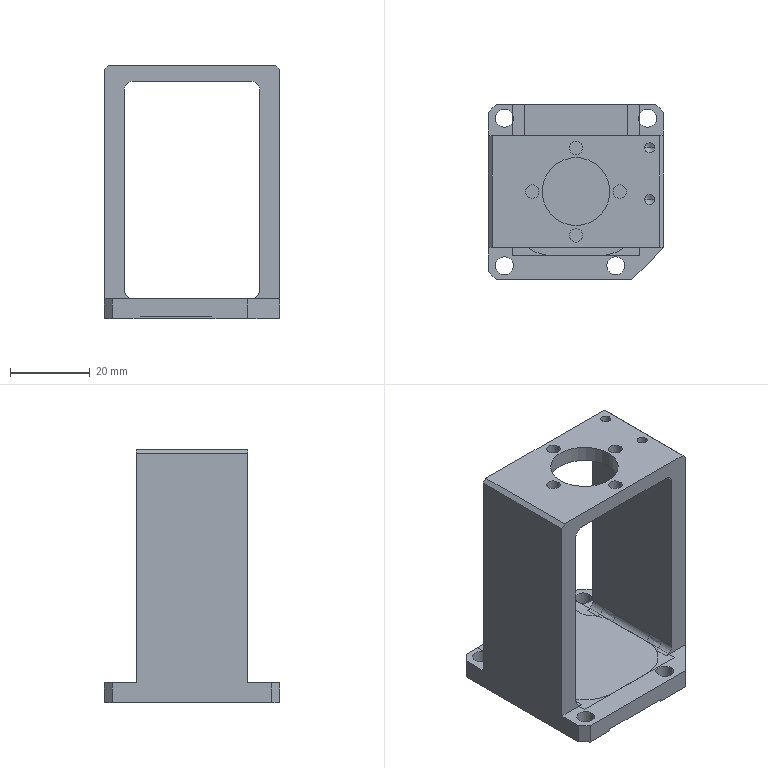NC program | NX | posted with a generic post | part box 44 x 44 x 63.6 mm
Lines 62 to 1050 of 4011:
(ZLEVEL_PROFILE , TOOL : D20)
N104 T02 M6
N106 G54
N108 G17 G0 G90 X0.611 Y32.1 B0. C0. S9500 M3
N110 G43 Z30. H2
N112 Z1.5
N114 G94 G1 X20.779 Z0.443 F1000.
N116 X22.872 Y31.714 Z0.332
N118 X24.838 Y30.9 Z0.22
N120 X26.591 Y29.693 Z0.108
N122 X29.693 Y26.591 Z-0.121
N124 X30.9 Y24.838 Z-0.233
N126 X31.714 Y22.872 Z-0.345
N128 X32.1 Y20.779 Z-0.456
N130 Y20. Z-0.497
N132 Y-20. F3000.
N134 G2 X29.142 Y-27.142 R10.1
N136 G1 X27.142 Y-29.142
N138 G2 X20. Y-32.1 R10.1
N140 G1 X-20.
N142 G2 X-27.142 Y-29.142 R10.1
N144 G1 X-29.142 Y-27.142
N146 G2 X-32.1 Y-20. R10.1
N148 G1 Y14.
N150 G2 X-29.142 Y21.142 R10.1
N152 G1 X-21.142 Y29.142
N154 G2 X-14. Y32.1 R10.1
N156 G1 X20.
N158 G2 X27.142 Y29.142 R10.1
N160 G1 X29.142 Y27.142
N162 G2 X32.1 Y20. R10.1
N164 G1 Y-8.466 Z-0.994
N166 Y-20.
N168 G2 X29.142 Y-27.142 R10.1
N170 G1 X27.142 Y-29.142
N172 G2 X20. Y-32.1 R10.1
N174 G1 X-20.
N176 G2 X-27.142 Y-29.142 R10.1
N178 G1 X-29.142 Y-27.142
N180 G2 X-32.1 Y-20. R10.1
N182 G1 Y14.
N184 G2 X-29.142 Y21.142 R10.1
N186 G1 X-21.142 Y29.142
N188 G2 X-14. Y32.1 R10.1
N190 G1 X20.
N192 G2 X27.142 Y29.142 R10.1
N194 G1 X29.142 Y27.142
N196 G2 X32.1 Y20. R10.1
N198 G1 Y-8.466 Z-1.491
N200 Y-20.
N202 G2 X29.142 Y-27.142 R10.1
N204 G1 X27.142 Y-29.142
N206 G2 X20. Y-32.1 R10.1
N208 G1 X-20.
N210 G2 X-27.142 Y-29.142 R10.1
N212 G1 X-29.142 Y-27.142
N214 G2 X-32.1 Y-20. R10.1
N216 G1 Y14.
N218 G2 X-29.142 Y21.142 R10.1
N220 G1 X-21.142 Y29.142
N222 G2 X-14. Y32.1 R10.1
N224 G1 X20.
N226 G2 X27.142 Y29.142 R10.1
N228 G1 X29.142 Y27.142
N230 G2 X32.1 Y20. R10.1
N232 G1 Y-8.466 Z-1.988
N234 Y-20.
N236 G2 X29.142 Y-27.142 R10.1
N238 G1 X27.142 Y-29.142
N240 G2 X20. Y-32.1 R10.1
N242 G1 X-20.
N244 G2 X-27.142 Y-29.142 R10.1
N246 G1 X-29.142 Y-27.142
N248 G2 X-32.1 Y-20. R10.1
N250 G1 Y14.
N252 G2 X-29.142 Y21.142 R10.1
N254 G1 X-21.142 Y29.142
N256 G2 X-14. Y32.1 R10.1
N258 G1 X20.
N260 G2 X27.142 Y29.142 R10.1
N262 G1 X29.142 Y27.142
N264 G2 X32.1 Y20. R10.1
N266 G1 Y-8.466 Z-2.484
N268 Y-20.
N270 G2 X29.142 Y-27.142 R10.1
N272 G1 X27.142 Y-29.142
N274 G2 X20. Y-32.1 R10.1
N276 G1 X-20.
N278 G2 X-27.142 Y-29.142 R10.1
N280 G1 X-29.142 Y-27.142
N282 G2 X-32.1 Y-20. R10.1
N284 G1 Y14.
N286 G2 X-29.142 Y21.142 R10.1
N288 G1 X-21.142 Y29.142
N290 G2 X-14. Y32.1 R10.1
N292 G1 X20.
N294 G2 X27.142 Y29.142 R10.1
N296 G1 X29.142 Y27.142
N298 G2 X32.1 Y20. R10.1
N300 G1 Y-8.466 Z-2.981
N302 Y-20.
N304 G2 X29.142 Y-27.142 R10.1
N306 G1 X27.142 Y-29.142
N308 G2 X20. Y-32.1 R10.1
N310 G1 X-20.
N312 G2 X-27.142 Y-29.142 R10.1
N314 G1 X-29.142 Y-27.142
N316 G2 X-32.1 Y-20. R10.1
N318 G1 Y14.
N320 G2 X-29.142 Y21.142 R10.1
N322 G1 X-21.142 Y29.142
N324 G2 X-14. Y32.1 R10.1
N326 G1 X20.
N328 G2 X27.142 Y29.142 R10.1
N330 G1 X29.142 Y27.142
N332 G2 X32.1 Y20. R10.1
N334 G1 Y-8.466 Z-3.478
N336 Y-20.
N338 G2 X29.142 Y-27.142 R10.1
N340 G1 X27.142 Y-29.142
N342 G2 X20. Y-32.1 R10.1
N344 G1 X-20.
N346 G2 X-27.142 Y-29.142 R10.1
N348 G1 X-29.142 Y-27.142
N350 G2 X-32.1 Y-20. R10.1
N352 G1 Y14.
N354 G2 X-29.142 Y21.142 R10.1
N356 G1 X-21.142 Y29.142
N358 G2 X-14. Y32.1 R10.1
N360 G1 X20.
N362 G2 X27.142 Y29.142 R10.1
N364 G1 X29.142 Y27.142
N366 G2 X32.1 Y20. R10.1
N368 G1 Y-8.466 Z-3.975
N370 Y-20.
N372 G2 X29.142 Y-27.142 R10.1
N374 G1 X27.142 Y-29.142
N376 G2 X20. Y-32.1 R10.1
N378 G1 X-20.
N380 G2 X-27.142 Y-29.142 R10.1
N382 G1 X-29.142 Y-27.142
N384 G2 X-32.1 Y-20. R10.1
N386 G1 Y14.
N388 G2 X-29.142 Y21.142 R10.1
N390 G1 X-21.142 Y29.142
N392 G2 X-14. Y32.1 R10.1
N394 G1 X20.
N396 G2 X27.142 Y29.142 R10.1
N398 G1 X29.142 Y27.142
N400 G2 X32.1 Y20. R10.1
N402 G1 Y-8.466 Z-4.472
N404 Y-20.
N406 G2 X29.142 Y-27.142 R10.1
N408 G1 X27.142 Y-29.142
N410 G2 X20. Y-32.1 R10.1
N412 G1 X-20.
N414 G2 X-27.142 Y-29.142 R10.1
N416 G1 X-29.142 Y-27.142
N418 G2 X-32.1 Y-20. R10.1
N420 G1 Y14.
N422 G2 X-29.142 Y21.142 R10.1
N424 G1 X-21.142 Y29.142
N426 G2 X-14. Y32.1 R10.1
N428 G1 X20.
N430 G2 X27.142 Y29.142 R10.1
N432 G1 X29.142 Y27.142
N434 G2 X32.1 Y20. R10.1
N436 G1 Y-8.466 Z-4.969
N438 Y-20.
N440 G2 X29.142 Y-27.142 R10.1
N442 G1 X27.142 Y-29.142
N444 G2 X20. Y-32.1 R10.1
N446 G1 X-20.
N448 G2 X-27.142 Y-29.142 R10.1
N450 G1 X-29.142 Y-27.142
N452 G2 X-32.1 Y-20. R10.1
N454 G1 Y14.
N456 G2 X-29.142 Y21.142 R10.1
N458 G1 X-21.142 Y29.142
N460 G2 X-14. Y32.1 R10.1
N462 G1 X20.
N464 G2 X27.142 Y29.142 R10.1
N466 G1 X29.142 Y27.142
N468 G2 X32.1 Y20. R10.1
N470 G1 Y-8.466 Z-5.466
N472 Y-20.
N474 G2 X29.142 Y-27.142 R10.1
N476 G1 X27.142 Y-29.142
N478 G2 X20. Y-32.1 R10.1
N480 G1 X-20.
N482 G2 X-27.142 Y-29.142 R10.1
N484 G1 X-29.142 Y-27.142
N486 G2 X-32.1 Y-20. R10.1
N488 G1 Y14.
N490 G2 X-29.142 Y21.142 R10.1
N492 G1 X-21.142 Y29.142
N494 G2 X-14. Y32.1 R10.1
N496 G1 X20.
N498 G2 X27.142 Y29.142 R10.1
N500 G1 X29.142 Y27.142
N502 G2 X32.1 Y20. R10.1
N504 G1 Y-8.466 Z-5.963
N506 Y-20.
N508 G2 X29.142 Y-27.142 R10.1
N510 G1 X27.142 Y-29.142
N512 G2 X20. Y-32.1 R10.1
N514 G1 X-20.
N516 G2 X-27.142 Y-29.142 R10.1
N518 G1 X-29.142 Y-27.142
N520 G2 X-32.1 Y-20. R10.1
N522 G1 Y14.
N524 G2 X-29.142 Y21.142 R10.1
N526 G1 X-21.142 Y29.142
N528 G2 X-14. Y32.1 R10.1
N530 G1 X20.
N532 G2 X27.142 Y29.142 R10.1
N534 G1 X29.142 Y27.142
N536 G2 X32.1 Y20. R10.1
N538 G1 Y-8.466 Z-6.459
N540 Y-20.
N542 G2 X29.142 Y-27.142 R10.1
N544 G1 X27.142 Y-29.142
N546 G2 X20. Y-32.1 R10.1
N548 G1 X-20.
N550 G2 X-27.142 Y-29.142 R10.1
N552 G1 X-29.142 Y-27.142
N554 G2 X-32.1 Y-20. R10.1
N556 G1 Y14.
N558 G2 X-29.142 Y21.142 R10.1
N560 G1 X-21.142 Y29.142
N562 G2 X-14. Y32.1 R10.1
N564 G1 X20.
N566 G2 X27.142 Y29.142 R10.1
N568 G1 X29.142 Y27.142
N570 G2 X32.1 Y20. R10.1
N572 G1 Y-8.466 Z-6.956
N574 Y-20.
N576 G2 X29.142 Y-27.142 R10.1
N578 G1 X27.142 Y-29.142
N580 G2 X20. Y-32.1 R10.1
N582 G1 X-20.
N584 G2 X-27.142 Y-29.142 R10.1
N586 G1 X-29.142 Y-27.142
N588 G2 X-32.1 Y-20. R10.1
N590 G1 Y14.
N592 G2 X-29.142 Y21.142 R10.1
N594 G1 X-21.142 Y29.142
N596 G2 X-14. Y32.1 R10.1
N598 G1 X20.
N600 G2 X27.142 Y29.142 R10.1
N602 G1 X29.142 Y27.142
N604 G2 X32.1 Y20. R10.1
N606 G1 Y-8.466 Z-7.453
N608 Y-20.
N610 G2 X29.142 Y-27.142 R10.1
N612 G1 X27.142 Y-29.142
N614 G2 X20. Y-32.1 R10.1
N616 G1 X-20.
N618 G2 X-27.142 Y-29.142 R10.1
N620 G1 X-29.142 Y-27.142
N622 G2 X-32.1 Y-20. R10.1
N624 G1 Y14.
N626 G2 X-29.142 Y21.142 R10.1
N628 G1 X-21.142 Y29.142
N630 G2 X-14. Y32.1 R10.1
N632 G1 X20.
N634 G2 X27.142 Y29.142 R10.1
N636 G1 X29.142 Y27.142
N638 G2 X32.1 Y20. R10.1
N640 G1 Y-8.466 Z-7.95
N642 Y-20.
N644 G2 X29.142 Y-27.142 R10.1
N646 G1 X27.142 Y-29.142
N648 G2 X20. Y-32.1 R10.1
N650 G1 X-20.
N652 G2 X-27.142 Y-29.142 R10.1
N654 G1 X-29.142 Y-27.142
N656 G2 X-32.1 Y-20. R10.1
N658 G1 Y14.
N660 G2 X-29.142 Y21.142 R10.1
N662 G1 X-21.142 Y29.142
N664 G2 X-14. Y32.1 R10.1
N666 G1 X20.
N668 G2 X27.142 Y29.142 R10.1
N670 G1 X29.142 Y27.142
N672 G2 X32.1 Y20. R10.1
N674 G1 Y-8.466 Z-8.447
N676 Y-20.
N678 G2 X29.142 Y-27.142 R10.1
N680 G1 X27.142 Y-29.142
N682 G2 X20. Y-32.1 R10.1
N684 G1 X-20.
N686 G2 X-27.142 Y-29.142 R10.1
N688 G1 X-29.142 Y-27.142
N690 G2 X-32.1 Y-20. R10.1
N692 G1 Y14.
N694 G2 X-29.142 Y21.142 R10.1
N696 G1 X-21.142 Y29.142
N698 G2 X-14. Y32.1 R10.1
N700 G1 X20.
N702 G2 X27.142 Y29.142 R10.1
N704 G1 X29.142 Y27.142
N706 G2 X32.1 Y20. R10.1
N708 G1 Y-8.466 Z-8.944
N710 Y-20.
N712 G2 X29.142 Y-27.142 R10.1
N714 G1 X27.142 Y-29.142
N716 G2 X20. Y-32.1 R10.1
N718 G1 X-20.
N720 G2 X-27.142 Y-29.142 R10.1
N722 G1 X-29.142 Y-27.142
N724 G2 X-32.1 Y-20. R10.1
N726 G1 Y14.
N728 G2 X-29.142 Y21.142 R10.1
N730 G1 X-21.142 Y29.142
N732 G2 X-14. Y32.1 R10.1
N734 G1 X20.
N736 G2 X27.142 Y29.142 R10.1
N738 G1 X29.142 Y27.142
N740 G2 X32.1 Y20. R10.1
N742 G1 Y-8.466 Z-9.441
N744 Y-20.
N746 G2 X29.142 Y-27.142 R10.1
N748 G1 X27.142 Y-29.142
N750 G2 X20. Y-32.1 R10.1
N752 G1 X-20.
N754 G2 X-27.142 Y-29.142 R10.1
N756 G1 X-29.142 Y-27.142
N758 G2 X-32.1 Y-20. R10.1
N760 G1 Y14.
N762 G2 X-29.142 Y21.142 R10.1
N764 G1 X-21.142 Y29.142
N766 G2 X-14. Y32.1 R10.1
N768 G1 X20.
N770 G2 X27.142 Y29.142 R10.1
N772 G1 X29.142 Y27.142
N774 G2 X32.1 Y20. R10.1
N776 G1 Y-8.466 Z-9.938
N778 Y-20.
N780 G2 X29.142 Y-27.142 R10.1
N782 G1 X27.142 Y-29.142
N784 G2 X20. Y-32.1 R10.1
N786 G1 X-20.
N788 G2 X-27.142 Y-29.142 R10.1
N790 G1 X-29.142 Y-27.142
N792 G2 X-32.1 Y-20. R10.1
N794 G1 Y14.
N796 G2 X-29.142 Y21.142 R10.1
N798 G1 X-21.142 Y29.142
N800 G2 X-14. Y32.1 R10.1
N802 G1 X20.
N804 G2 X27.142 Y29.142 R10.1
N806 G1 X29.142 Y27.142
N808 G2 X32.1 Y20. R10.1
N810 G1 Y-8.466 Z-10.434
N812 Y-20.
N814 G2 X29.142 Y-27.142 R10.1
N816 G1 X27.142 Y-29.142
N818 G2 X20. Y-32.1 R10.1
N820 G1 X-20.
N822 G2 X-27.142 Y-29.142 R10.1
N824 G1 X-29.142 Y-27.142
N826 G2 X-32.1 Y-20. R10.1
N828 G1 Y14.
N830 G2 X-29.142 Y21.142 R10.1
N832 G1 X-21.142 Y29.142
N834 G2 X-14. Y32.1 R10.1
N836 G1 X20.
N838 G2 X27.142 Y29.142 R10.1
N840 G1 X29.142 Y27.142
N842 G2 X32.1 Y20. R10.1
N844 G1 Y-8.466 Z-10.931
N846 Y-20.
N848 G2 X29.142 Y-27.142 R10.1
N850 G1 X27.142 Y-29.142
N852 G2 X20. Y-32.1 R10.1
N854 G1 X-20.
N856 G2 X-27.142 Y-29.142 R10.1
N858 G1 X-29.142 Y-27.142
N860 G2 X-32.1 Y-20. R10.1
N862 G1 Y14.
N864 G2 X-29.142 Y21.142 R10.1
N866 G1 X-21.142 Y29.142
N868 G2 X-14. Y32.1 R10.1
N870 G1 X20.
N872 G2 X27.142 Y29.142 R10.1
N874 G1 X29.142 Y27.142
N876 G2 X32.1 Y20. R10.1
N878 G1 Y-8.466 Z-11.428
N880 Y-20.
N882 G2 X29.142 Y-27.142 R10.1
N884 G1 X27.142 Y-29.142
N886 G2 X20. Y-32.1 R10.1
N888 G1 X-20.
N890 G2 X-27.142 Y-29.142 R10.1
N892 G1 X-29.142 Y-27.142
N894 G2 X-32.1 Y-20. R10.1
N896 G1 Y14.
N898 G2 X-29.142 Y21.142 R10.1
N900 G1 X-21.142 Y29.142
N902 G2 X-14. Y32.1 R10.1
N904 G1 X20.
N906 G2 X27.142 Y29.142 R10.1
N908 G1 X29.142 Y27.142
N910 G2 X32.1 Y20. R10.1
N912 G1 Y-8.466 Z-11.925
N914 Y-20.
N916 G2 X29.142 Y-27.142 R10.1
N918 G1 X27.142 Y-29.142
N920 G2 X20. Y-32.1 R10.1
N922 G1 X-20.
N924 G2 X-27.142 Y-29.142 R10.1
N926 G1 X-29.142 Y-27.142
N928 G2 X-32.1 Y-20. R10.1
N930 G1 Y14.
N932 G2 X-29.142 Y21.142 R10.1
N934 G1 X-21.142 Y29.142
N936 G2 X-14. Y32.1 R10.1
N938 G1 X20.
N940 G2 X27.142 Y29.142 R10.1
N942 G1 X29.142 Y27.142
N944 G2 X32.1 Y20. R10.1
N946 G1 Y-8.466 Z-12.422
N948 Y-20.
N950 G2 X29.142 Y-27.142 R10.1
N952 G1 X27.142 Y-29.142
N954 G2 X20. Y-32.1 R10.1
N956 G1 X-20.
N958 G2 X-27.142 Y-29.142 R10.1
N960 G1 X-29.142 Y-27.142
N962 G2 X-32.1 Y-20. R10.1
N964 G1 Y14.
N966 G2 X-29.142 Y21.142 R10.1
N968 G1 X-21.142 Y29.142
N970 G2 X-14. Y32.1 R10.1
N972 G1 X20.
N974 G2 X27.142 Y29.142 R10.1
N976 G1 X29.142 Y27.142
N978 G2 X32.1 Y20. R10.1
N980 G1 Y-8.466 Z-12.919
N982 Y-20.
N984 G2 X29.142 Y-27.142 R10.1
N986 G1 X27.142 Y-29.142
N988 G2 X20. Y-32.1 R10.1
N990 G1 X-20.
N992 G2 X-27.142 Y-29.142 R10.1
N994 G1 X-29.142 Y-27.142
N996 G2 X-32.1 Y-20. R10.1
N998 G1 Y14.
N1000 G2 X-29.142 Y21.142 R10.1
N1002 G1 X-21.142 Y29.142
N1004 G2 X-14. Y32.1 R10.1
N1006 G1 X20.
N1008 G2 X27.142 Y29.142 R10.1
N1010 G1 X29.142 Y27.142
N1012 G2 X32.1 Y20. R10.1
N1014 G1 Y-8.466 Z-13.416
N1016 Y-20.
N1018 G2 X29.142 Y-27.142 R10.1
N1020 G1 X27.142 Y-29.142
N1022 G2 X20. Y-32.1 R10.1
N1024 G1 X-20.
N1026 G2 X-27.142 Y-29.142 R10.1
N1028 G1 X-29.142 Y-27.142
N1030 G2 X-32.1 Y-20. R10.1
N1032 G1 Y14.
N1034 G2 X-29.142 Y21.142 R10.1
N1036 G1 X-21.142 Y29.142
N1038 G2 X-14. Y32.1 R10.1
N1040 G1 X20.
N1042 G2 X27.142 Y29.142 R10.1
N1044 G1 X29.142 Y27.142
N1046 G2 X32.1 Y20. R10.1
N1048 G1 Y-8.466 Z-13.913
N1050 Y-20.
N1052 G2 X29.142 Y-27.142 R10.1
N1054 G1 X27.142 Y-29.142
N1056 G2 X20. Y-32.1 R10.1
N1058 G1 X-20.
N1060 G2 X-27.142 Y-29.142 R10.1
N1062 G1 X-29.142 Y-27.142
N1064 G2 X-32.1 Y-20. R10.1
N1066 G1 Y14.
N1068 G2 X-29.142 Y21.142 R10.1
N1070 G1 X-21.142 Y29.142
N1072 G2 X-14. Y32.1 R10.1
N1074 G1 X20.
N1076 G2 X27.142 Y29.142 R10.1
N1078 G1 X29.142 Y27.142
N1080 G2 X32.1 Y20. R10.1
N1082 G1 Y-8.466 Z-14.409
N1084 Y-20.
N1086 G2 X29.142 Y-27.142 R10.1
N1088 G1 X27.142 Y-29.142
N1090 G2 X20. Y-32.1 R10.1
N1092 G1 X-20.
N1094 G2 X-27.142 Y-29.142 R10.1
N1096 G1 X-29.142 Y-27.142
N1098 G2 X-32.1 Y-20. R10.1
N1100 G1 Y14.
N1102 G2 X-29.142 Y21.142 R10.1
N1104 G1 X-21.142 Y29.142
N1106 G2 X-14. Y32.1 R10.1
N1108 G1 X20.
N1110 G2 X27.142 Y29.142 R10.1
N1112 G1 X29.142 Y27.142
N1114 G2 X32.1 Y20. R10.1
N1116 G1 Y-8.466 Z-14.906
N1118 Y-20.
N1120 G2 X29.142 Y-27.142 R10.1
N1122 G1 X27.142 Y-29.142
N1124 G2 X20. Y-32.1 R10.1
N1126 G1 X-20.
N1128 G2 X-27.142 Y-29.142 R10.1
N1130 G1 X-29.142 Y-27.142
N1132 G2 X-32.1 Y-20. R10.1
N1134 G1 Y14.
N1136 G2 X-29.142 Y21.142 R10.1
N1138 G1 X-21.142 Y29.142
N1140 G2 X-14. Y32.1 R10.1
N1142 G1 X20.
N1144 G2 X27.142 Y29.142 R10.1
N1146 G1 X29.142 Y27.142
N1148 G2 X32.1 Y20. R10.1
N1150 G1 Y-8.466 Z-15.403
N1152 Y-20.
N1154 G2 X29.142 Y-27.142 R10.1
N1156 G1 X27.142 Y-29.142
N1158 G2 X20. Y-32.1 R10.1
N1160 G1 X-20.
N1162 G2 X-27.142 Y-29.142 R10.1
N1164 G1 X-29.142 Y-27.142
N1166 G2 X-32.1 Y-20. R10.1
N1168 G1 Y14.
N1170 G2 X-29.142 Y21.142 R10.1
N1172 G1 X-21.142 Y29.142
N1174 G2 X-14. Y32.1 R10.1
N1176 G1 X20.
N1178 G2 X27.142 Y29.142 R10.1
N1180 G1 X29.142 Y27.142
N1182 G2 X32.1 Y20. R10.1
N1184 G1 Y-8.466 Z-15.9
N1186 Y-20.
N1188 G2 X29.142 Y-27.142 R10.1
N1190 G1 X27.142 Y-29.142
N1192 G2 X20. Y-32.1 R10.1
N1194 G1 X-20.
N1196 G2 X-27.142 Y-29.142 R10.1
N1198 G1 X-29.142 Y-27.142
N1200 G2 X-32.1 Y-20. R10.1
N1202 G1 Y14.
N1204 G2 X-29.142 Y21.142 R10.1
N1206 G1 X-21.142 Y29.142
N1208 G2 X-14. Y32.1 R10.1
N1210 G1 X20.
N1212 G2 X27.142 Y29.142 R10.1
N1214 G1 X29.142 Y27.142
N1216 G2 X32.1 Y20. R10.1
N1218 G1 Y-8.466 Z-16.397
N1220 Y-20.
N1222 G2 X29.142 Y-27.142 R10.1
N1224 G1 X27.142 Y-29.142
N1226 G2 X20. Y-32.1 R10.1
N1228 G1 X-20.
N1230 G2 X-27.142 Y-29.142 R10.1
N1232 G1 X-29.142 Y-27.142
N1234 G2 X-32.1 Y-20. R10.1
N1236 G1 Y14.
N1238 G2 X-29.142 Y21.142 R10.1
N1240 G1 X-21.142 Y29.142
N1242 G2 X-14. Y32.1 R10.1
N1244 G1 X20.
N1246 G2 X27.142 Y29.142 R10.1
N1248 G1 X29.142 Y27.142
N1250 G2 X32.1 Y20. R10.1
N1252 G1 Y-8.466 Z-16.894
N1254 Y-20.
N1256 G2 X29.142 Y-27.142 R10.1
N1258 G1 X27.142 Y-29.142
N1260 G2 X20. Y-32.1 R10.1
N1262 G1 X-20.
N1264 G2 X-27.142 Y-29.142 R10.1
N1266 G1 X-29.142 Y-27.142
N1268 G2 X-32.1 Y-20. R10.1
N1270 G1 Y14.
N1272 G2 X-29.142 Y21.142 R10.1
N1274 G1 X-21.142 Y29.142
N1276 G2 X-14. Y32.1 R10.1
N1278 G1 X20.
N1280 G2 X27.142 Y29.142 R10.1
N1282 G1 X29.142 Y27.142
N1284 G2 X32.1 Y20. R10.1
N1286 G1 Y-8.466 Z-17.391
N1288 Y-20.
N1290 G2 X29.142 Y-27.142 R10.1
N1292 G1 X27.142 Y-29.142
N1294 G2 X20. Y-32.1 R10.1
N1296 G1 X-20.
N1298 G2 X-27.142 Y-29.142 R10.1
N1300 G1 X-29.142 Y-27.142
N1302 G2 X-32.1 Y-20. R10.1
N1304 G1 Y14.
N1306 G2 X-29.142 Y21.142 R10.1
N1308 G1 X-21.142 Y29.142
N1310 G2 X-14. Y32.1 R10.1
N1312 G1 X20.
N1314 G2 X27.142 Y29.142 R10.1
N1316 G1 X29.142 Y27.142
N1318 G2 X32.1 Y20. R10.1
N1320 G1 Y-8.466 Z-17.888
N1322 Y-20.
N1324 G2 X29.142 Y-27.142 R10.1
N1326 G1 X27.142 Y-29.142
N1328 G2 X20. Y-32.1 R10.1
N1330 G1 X-20.
N1332 G2 X-27.142 Y-29.142 R10.1
N1334 G1 X-29.142 Y-27.142
N1336 G2 X-32.1 Y-20. R10.1
N1338 G1 Y14.
N1340 G2 X-29.142 Y21.142 R10.1
N1342 G1 X-21.142 Y29.142
N1344 G2 X-14. Y32.1 R10.1
N1346 G1 X20.
N1348 G2 X27.142 Y29.142 R10.1
N1350 G1 X29.142 Y27.142
N1352 G2 X32.1 Y20. R10.1
N1354 G1 Y-8.466 Z-18.384
N1356 Y-20.
N1358 G2 X29.142 Y-27.142 R10.1
N1360 G1 X27.142 Y-29.142
N1362 G2 X20. Y-32.1 R10.1
N1364 G1 X-20.
N1366 G2 X-27.142 Y-29.142 R10.1
N1368 G1 X-29.142 Y-27.142
N1370 G2 X-32.1 Y-20. R10.1
N1372 G1 Y14.
N1374 G2 X-29.142 Y21.142 R10.1
N1376 G1 X-21.142 Y29.142
N1378 G2 X-14. Y32.1 R10.1
N1380 G1 X20.
N1382 G2 X27.142 Y29.142 R10.1
N1384 G1 X29.142 Y27.142
N1386 G2 X32.1 Y20. R10.1
N1388 G1 Y-8.466 Z-18.881
N1390 Y-20.
N1392 G2 X29.142 Y-27.142 R10.1
N1394 G1 X27.142 Y-29.142
N1396 G2 X20. Y-32.1 R10.1
N1398 G1 X-20.
N1400 G2 X-27.142 Y-29.142 R10.1
N1402 G1 X-29.142 Y-27.142
N1404 G2 X-32.1 Y-20. R10.1
N1406 G1 Y14.
N1408 G2 X-29.142 Y21.142 R10.1
N1410 G1 X-21.142 Y29.142
N1412 G2 X-14. Y32.1 R10.1
N1414 G1 X20.
N1416 G2 X27.142 Y29.142 R10.1
N1418 G1 X29.142 Y27.142
N1420 G2 X32.1 Y20. R10.1
N1422 G1 Y-8.466 Z-19.378
N1424 Y-20.
N1426 G2 X29.142 Y-27.142 R10.1
N1428 G1 X27.142 Y-29.142
N1430 G2 X20. Y-32.1 R10.1
N1432 G1 X-20.
N1434 G2 X-27.142 Y-29.142 R10.1
N1436 G1 X-29.142 Y-27.142
N1438 G2 X-32.1 Y-20. R10.1
N1440 G1 Y14.
N1442 G2 X-29.142 Y21.142 R10.1
N1444 G1 X-21.142 Y29.142
N1446 G2 X-14. Y32.1 R10.1
N1448 G1 X20.
N1450 G2 X27.142 Y29.142 R10.1
N1452 G1 X29.142 Y27.142
N1454 G2 X32.1 Y20. R10.1
N1456 G1 Y-8.466 Z-19.875
N1458 Y-20.
N1460 G2 X29.142 Y-27.142 R10.1
N1462 G1 X27.142 Y-29.142
N1464 G2 X20. Y-32.1 R10.1
N1466 G1 X-20.
N1468 G2 X-27.142 Y-29.142 R10.1
N1470 G1 X-29.142 Y-27.142
N1472 G2 X-32.1 Y-20. R10.1
N1474 G1 Y14.
N1476 G2 X-29.142 Y21.142 R10.1
N1478 G1 X-21.142 Y29.142
N1480 G2 X-14. Y32.1 R10.1
N1482 G1 X20.
N1484 G2 X27.142 Y29.142 R10.1
N1486 G1 X29.142 Y27.142
N1488 G2 X32.1 Y20. R10.1
N1490 G1 Y-8.466 Z-20.372
N1492 Y-20.
N1494 G2 X29.142 Y-27.142 R10.1
N1496 G1 X27.142 Y-29.142
N1498 G2 X20. Y-32.1 R10.1
N1500 G1 X-20.
N1502 G2 X-27.142 Y-29.142 R10.1
N1504 G1 X-29.142 Y-27.142
N1506 G2 X-32.1 Y-20. R10.1
N1508 G1 Y14.
N1510 G2 X-29.142 Y21.142 R10.1
N1512 G1 X-21.142 Y29.142
N1514 G2 X-14. Y32.1 R10.1
N1516 G1 X20.
N1518 G2 X27.142 Y29.142 R10.1
N1520 G1 X29.142 Y27.142
N1522 G2 X32.1 Y20. R10.1
N1524 G1 Y-8.466 Z-20.869
N1526 Y-20.
N1528 G2 X29.142 Y-27.142 R10.1
N1530 G1 X27.142 Y-29.142
N1532 G2 X20. Y-32.1 R10.1
N1534 G1 X-20.
N1536 G2 X-27.142 Y-29.142 R10.1
N1538 G1 X-29.142 Y-27.142
N1540 G2 X-32.1 Y-20. R10.1
N1542 G1 Y14.
N1544 G2 X-29.142 Y21.142 R10.1
N1546 G1 X-21.142 Y29.142
N1548 G2 X-14. Y32.1 R10.1
N1550 G1 X20.
N1552 G2 X27.142 Y29.142 R10.1
N1554 G1 X29.142 Y27.142
N1556 G2 X32.1 Y20. R10.1
N1558 G1 Y-8.466 Z-21.366
N1560 Y-20.
N1562 G2 X29.142 Y-27.142 R10.1
N1564 G1 X27.142 Y-29.142
N1566 G2 X20. Y-32.1 R10.1
N1568 G1 X-20.
N1570 G2 X-27.142 Y-29.142 R10.1
N1572 G1 X-29.142 Y-27.142
N1574 G2 X-32.1 Y-20. R10.1
N1576 G1 Y14.
N1578 G2 X-29.142 Y21.142 R10.1
N1580 G1 X-21.142 Y29.142
N1582 G2 X-14. Y32.1 R10.1
N1584 G1 X20.
N1586 G2 X27.142 Y29.142 R10.1
N1588 G1 X29.142 Y27.142
N1590 G2 X32.1 Y20. R10.1
N1592 G1 Y-8.466 Z-21.863
N1594 Y-20.
N1596 G2 X29.142 Y-27.142 R10.1
N1598 G1 X27.142 Y-29.142
N1600 G2 X20. Y-32.1 R10.1
N1602 G1 X-20.
N1604 G2 X-27.142 Y-29.142 R10.1
N1606 G1 X-29.142 Y-27.142
N1608 G2 X-32.1 Y-20. R10.1
N1610 G1 Y14.
N1612 G2 X-29.142 Y21.142 R10.1
N1614 G1 X-21.142 Y29.142
N1616 G2 X-14. Y32.1 R10.1
N1618 G1 X20.
N1620 G2 X27.142 Y29.142 R10.1
N1622 G1 X29.142 Y27.142
N1624 G2 X32.1 Y20. R10.1
N1626 G1 Y-8.466 Z-22.359
N1628 Y-20.
N1630 G2 X29.142 Y-27.142 R10.1
N1632 G1 X27.142 Y-29.142
N1634 G2 X20. Y-32.1 R10.1
N1636 G1 X-20.
N1638 G2 X-27.142 Y-29.142 R10.1
N1640 G1 X-29.142 Y-27.142
N1642 G2 X-32.1 Y-20. R10.1
N1644 G1 Y14.
N1646 G2 X-29.142 Y21.142 R10.1
N1648 G1 X-21.142 Y29.142
N1650 G2 X-14. Y32.1 R10.1
N1652 G1 X20.
N1654 G2 X27.142 Y29.142 R10.1
N1656 G1 X29.142 Y27.142
N1658 G2 X32.1 Y20. R10.1
N1660 G1 Y-8.466 Z-22.856
N1662 Y-20.
N1664 G2 X29.142 Y-27.142 R10.1
N1666 G1 X27.142 Y-29.142
N1668 G2 X20. Y-32.1 R10.1
N1670 G1 X-20.
N1672 G2 X-27.142 Y-29.142 R10.1
N1674 G1 X-29.142 Y-27.142
N1676 G2 X-32.1 Y-20. R10.1
N1678 G1 Y14.
N1680 G2 X-29.142 Y21.142 R10.1
N1682 G1 X-21.142 Y29.142
N1684 G2 X-14. Y32.1 R10.1
N1686 G1 X20.
N1688 G2 X27.142 Y29.142 R10.1
N1690 G1 X29.142 Y27.142
N1692 G2 X32.1 Y20. R10.1
N1694 G1 Y-8.466 Z-23.353
N1696 Y-20.
N1698 G2 X29.142 Y-27.142 R10.1
N1700 G1 X27.142 Y-29.142
N1702 G2 X20. Y-32.1 R10.1
N1704 G1 X-20.
N1706 G2 X-27.142 Y-29.142 R10.1
N1708 G1 X-29.142 Y-27.142
N1710 G2 X-32.1 Y-20. R10.1
N1712 G1 Y14.
N1714 G2 X-29.142 Y21.142 R10.1
N1716 G1 X-21.142 Y29.142
N1718 G2 X-14. Y32.1 R10.1
N1720 G1 X20.
N1722 G2 X27.142 Y29.142 R10.1
N1724 G1 X29.142 Y27.142
N1726 G2 X32.1 Y20. R10.1
N1728 G1 Y-8.466 Z-23.85
N1730 Y-20.
N1732 G2 X29.142 Y-27.142 R10.1
N1734 G1 X27.142 Y-29.142
N1736 G2 X20. Y-32.1 R10.1
N1738 G1 X-20.
N1740 G2 X-27.142 Y-29.142 R10.1
N1742 G1 X-29.142 Y-27.142
N1744 G2 X-32.1 Y-20. R10.1
N1746 G1 Y14.
N1748 G2 X-29.142 Y21.142 R10.1
N1750 G1 X-21.142 Y29.142
N1752 G2 X-14. Y32.1 R10.1
N1754 G1 X20.
N1756 G2 X27.142 Y29.142 R10.1
N1758 G1 X29.142 Y27.142
N1760 G2 X32.1 Y20. R10.1
N1762 G1 Y-8.466 Z-24.347
N1764 Y-20.
N1766 G2 X29.142 Y-27.142 R10.1
N1768 G1 X27.142 Y-29.142
N1770 G2 X20. Y-32.1 R10.1
N1772 G1 X-20.
N1774 G2 X-27.142 Y-29.142 R10.1
N1776 G1 X-29.142 Y-27.142
N1778 G2 X-32.1 Y-20. R10.1
N1780 G1 Y14.
N1782 G2 X-29.142 Y21.142 R10.1
N1784 G1 X-21.142 Y29.142
N1786 G2 X-14. Y32.1 R10.1
N1788 G1 X20.
N1790 G2 X27.142 Y29.142 R10.1
N1792 G1 X29.142 Y27.142
N1794 G2 X32.1 Y20. R10.1
N1796 G1 Y-8.466 Z-24.844
N1798 Y-20.
N1800 G2 X29.142 Y-27.142 R10.1
N1802 G1 X27.142 Y-29.142
N1804 G2 X20. Y-32.1 R10.1
N1806 G1 X-20.
N1808 G2 X-27.142 Y-29.142 R10.1
N1810 G1 X-29.142 Y-27.142
N1812 G2 X-32.1 Y-20. R10.1
N1814 G1 Y14.
N1816 G2 X-29.142 Y21.142 R10.1
N1818 G1 X-21.142 Y29.142
N1820 G2 X-14. Y32.1 R10.1
N1822 G1 X20.
N1824 G2 X27.142 Y29.142 R10.1
N1826 G1 X29.142 Y27.142
N1828 G2 X32.1 Y20. R10.1
N1830 G1 Y-8.466 Z-25.341
N1832 Y-20.
N1834 G2 X29.142 Y-27.142 R10.1
N1836 G1 X27.142 Y-29.142
N1838 G2 X20. Y-32.1 R10.1
N1840 G1 X-20.
N1842 G2 X-27.142 Y-29.142 R10.1
N1844 G1 X-29.142 Y-27.142
N1846 G2 X-32.1 Y-20. R10.1
N1848 G1 Y14.
N1850 G2 X-29.142 Y21.142 R10.1
N1852 G1 X-21.142 Y29.142
N1854 G2 X-14. Y32.1 R10.1
N1856 G1 X20.
N1858 G2 X27.142 Y29.142 R10.1
N1860 G1 X29.142 Y27.142
N1862 G2 X32.1 Y20. R10.1
N1864 G1 Y-8.466 Z-25.838
N1866 Y-20.
N1868 G2 X29.142 Y-27.142 R10.1
N1870 G1 X27.142 Y-29.142
N1872 G2 X20. Y-32.1 R10.1
N1874 G1 X-20.
N1876 G2 X-27.142 Y-29.142 R10.1
N1878 G1 X-29.142 Y-27.142
N1880 G2 X-32.1 Y-20. R10.1
N1882 G1 Y14.
N1884 G2 X-29.142 Y21.142 R10.1
N1886 G1 X-21.142 Y29.142
N1888 G2 X-14. Y32.1 R10.1
N1890 G1 X20.
N1892 G2 X27.142 Y29.142 R10.1
N1894 G1 X29.142 Y27.142
N1896 G2 X32.1 Y20. R10.1
N1898 G1 Y-8.466 Z-26.334
N1900 Y-20.
N1902 G2 X29.142 Y-27.142 R10.1
N1904 G1 X27.142 Y-29.142
N1906 G2 X20. Y-32.1 R10.1
N1908 G1 X-20.
N1910 G2 X-27.142 Y-29.142 R10.1
N1912 G1 X-29.142 Y-27.142
N1914 G2 X-32.1 Y-20. R10.1
N1916 G1 Y14.
N1918 G2 X-29.142 Y21.142 R10.1
N1920 G1 X-21.142 Y29.142
N1922 G2 X-14. Y32.1 R10.1
N1924 G1 X20.
N1926 G2 X27.142 Y29.142 R10.1
N1928 G1 X29.142 Y27.142
N1930 G2 X32.1 Y20. R10.1
N1932 G1 Y-8.466 Z-26.831
N1934 Y-20.
N1936 G2 X29.142 Y-27.142 R10.1
N1938 G1 X27.142 Y-29.142
N1940 G2 X20. Y-32.1 R10.1
N1942 G1 X-20.
N1944 G2 X-27.142 Y-29.142 R10.1
N1946 G1 X-29.142 Y-27.142
N1948 G2 X-32.1 Y-20. R10.1
N1950 G1 Y14.
N1952 G2 X-29.142 Y21.142 R10.1
N1954 G1 X-21.142 Y29.142
N1956 G2 X-14. Y32.1 R10.1
N1958 G1 X20.
N1960 G2 X27.142 Y29.142 R10.1
N1962 G1 X29.142 Y27.142
N1964 G2 X32.1 Y20. R10.1
N1966 G1 Y-8.466 Z-27.328
N1968 Y-20.
N1970 G2 X29.142 Y-27.142 R10.1
N1972 G1 X27.142 Y-29.142
N1974 G2 X20. Y-32.1 R10.1
N1976 G1 X-20.
N1978 G2 X-27.142 Y-29.142 R10.1
N1980 G1 X-29.142 Y-27.142
N1982 G2 X-32.1 Y-20. R10.1
N1984 G1 Y14.
N1986 G2 X-29.142 Y21.142 R10.1
N1988 G1 X-21.142 Y29.142
N1990 G2 X-14. Y32.1 R10.1
N1992 G1 X20.
N1994 G2 X27.142 Y29.142 R10.1
N1996 G1 X29.142 Y27.142
N1998 G2 X32.1 Y20. R10.1
N2000 G1 Y-8.466 Z-27.825
N2002 Y-20.
N2004 G2 X29.142 Y-27.142 R10.1
N2006 G1 X27.142 Y-29.142
N2008 G2 X20. Y-32.1 R10.1
N2010 G1 X-20.
N2012 G2 X-27.142 Y-29.142 R10.1
N2014 G1 X-29.142 Y-27.142
N2016 G2 X-32.1 Y-20. R10.1
N2018 G1 Y14.
N2020 G2 X-29.142 Y21.142 R10.1
N2022 G1 X-21.142 Y29.142
N2024 G2 X-14. Y32.1 R10.1
N2026 G1 X20.
N2028 G2 X27.142 Y29.142 R10.1
N2030 G1 X29.142 Y27.142
N2032 G2 X32.1 Y20. R10.1
N2034 G1 Y-8.466 Z-28.322
N2036 Y-20.
N2038 G2 X29.142 Y-27.142 R10.1
N2040 G1 X27.142 Y-29.142
N2042 G2 X20. Y-32.1 R10.1
N2044 G1 X-20.
N2046 G2 X-27.142 Y-29.142 R10.1
N2048 G1 X-29.142 Y-27.142
N2050 G2 X-32.1 Y-20. R10.1
N2052 G1 Y14.
N2054 G2 X-29.142 Y21.142 R10.1
N2056 G1 X-21.142 Y29.142
N2058 G2 X-14. Y32.1 R10.1
N2060 G1 X20.
N2062 G2 X27.142 Y29.142 R10.1
N2064 G1 X29.142 Y27.142
N2066 G2 X32.1 Y20. R10.1
N2068 G1 Y-8.466 Z-28.819
N2070 Y-20.
N2072 G2 X29.142 Y-27.142 R10.1
N2074 G1 X27.142 Y-29.142